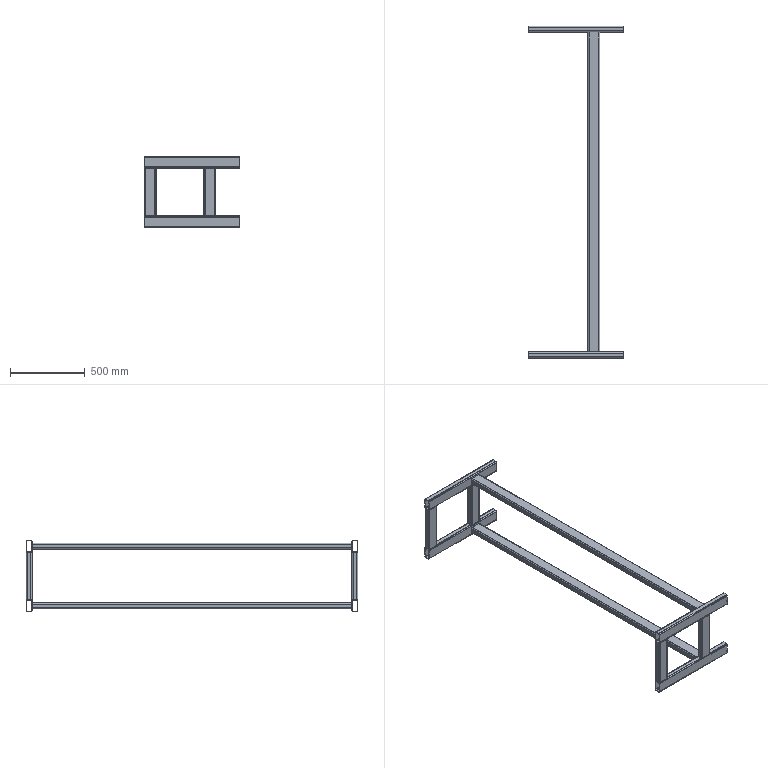Part | SolidWorks | features 3DProfileFeature 1, WeldMemberFeat 1, WeldmentFeature 1 | 10 solids | 180 faces | box 640 x 2220 x 480 mm | volume 6940947 mm3 | plane 100 | cylinder 80 | commonest cylinder face diameters 8 x40 16 x40